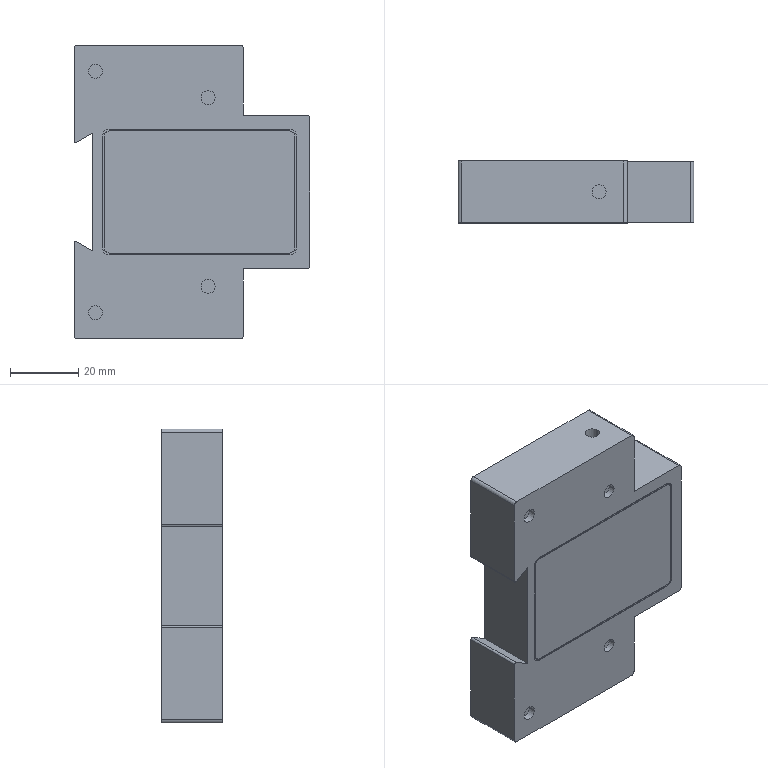Part | STEP file | 0008 | 1 solid | 126 faces | box 68.959 x 18 x 86 mm | volume 88648 mm3 | plane 74 | cylinder 52 | commonest cylinder face diameters 4.125 x20 3 x8 4 x8 2 x6 6.767 x4 7.167 x4